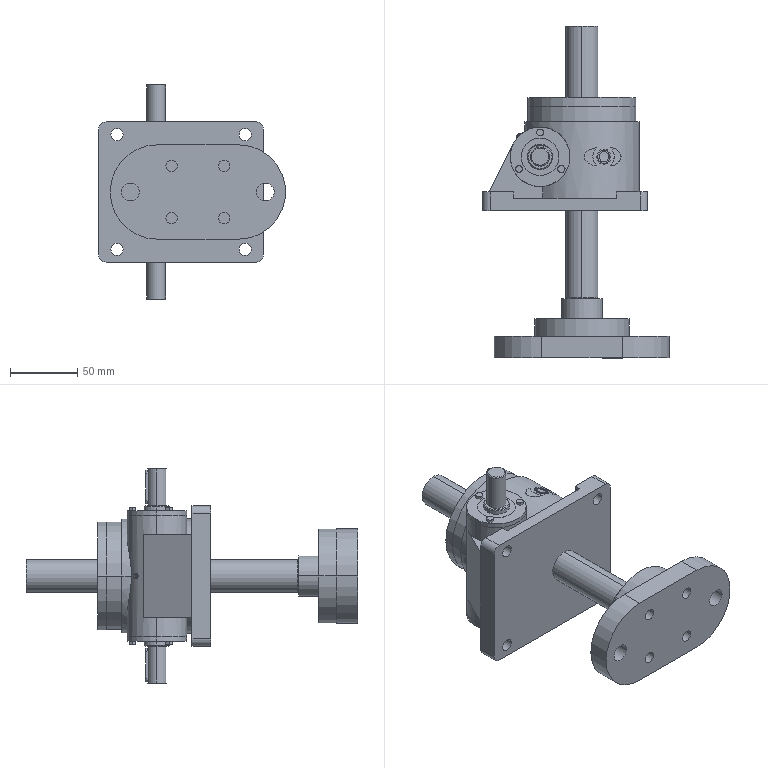Part | SolidWorks | 4 solids | 316 faces | box 138.5 x 246 x 160 mm | volume 888855 mm3 | plane 116 | cylinder 94 | cone 54 | spline 46 | torus 6 | commonest cylinder face diameters 8.5 x8 9 x8 10 x8 44.2 x7 5 x6 70 x5